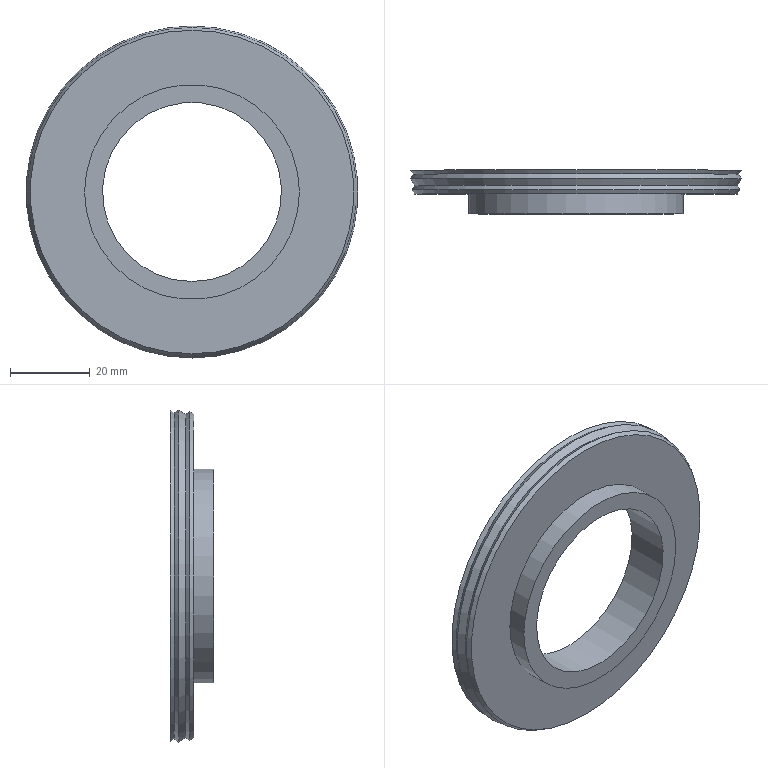Part | NX | features DATUM_CSYS 5, SKETCH 4, EXTRUDE 3, SWP104 1 | 1 solid | 10 faces | box 83.468 x 11 x 83.468 mm | volume 25904 mm3 | cone 5 | plane 3 | cylinder 2 | commonest cylinder face diameters 45 x1 54 x1
STEP:
#1=CARTESIAN_POINT('',(27.,-6.,0.));
#2=VERTEX_POINT('',#1);
#3=CARTESIAN_POINT('',(0.,-6.,0.));
#4=DIRECTION('',(0.,-1.,0.));
#5=DIRECTION('',(1.,0.,0.));
#6=AXIS2_PLACEMENT_3D('',#3,#4,#5);
#7=CIRCLE('',#6,27.);
#8=EDGE_CURVE('',#2,#2,#7,.T.);
#9=ORIENTED_EDGE('',*,*,#8,.F.);
#10=EDGE_LOOP('',(#9));
#11=FACE_BOUND('',#10,.T.);
#12=CARTESIAN_POINT('',(0.,-6.,-40.661));
#13=VERTEX_POINT('',#12);
#14=CARTESIAN_POINT('',(0.,-6.,0.));
#15=DIRECTION('',(0.,-1.,0.));
#16=DIRECTION('',(0.,0.,-1.));
#17=AXIS2_PLACEMENT_3D('',#14,#15,#16);
#18=CIRCLE('',#17,40.661);
#19=EDGE_CURVE('',#13,#13,#18,.T.);
#20=ORIENTED_EDGE('',*,*,#19,.T.);
#21=EDGE_LOOP('',(#20));
#22=FACE_BOUND('',#21,.T.);
#23=CARTESIAN_POINT('',(0.,-6.,0.));
#24=DIRECTION('',(0.,-1.,0.));
#25=DIRECTION('',(0.,0.,-1.));
#26=AXIS2_PLACEMENT_3D('',#23,#24,#25);
#27=PLANE('',#26);
#28=ADVANCED_FACE('',(#11,#22),#27,.T.);
#29=CARTESIAN_POINT('',(27.,-11.,0.));
#30=VERTEX_POINT('',#29);
#31=CARTESIAN_POINT('',(0.,-11.,0.));
#32=DIRECTION('',(0.,-1.,0.));
#33=DIRECTION('',(1.,0.,0.));
#34=AXIS2_PLACEMENT_3D('',#31,#32,#33);
#35=CIRCLE('',#34,27.);
#36=EDGE_CURVE('',#30,#30,#35,.T.);
#37=ORIENTED_EDGE('',*,*,#36,.F.);
#38=EDGE_LOOP('',(#37));
#39=FACE_BOUND('',#38,.T.);
#40=ORIENTED_EDGE('',*,*,#8,.T.);
#41=EDGE_LOOP('',(#40));
#42=FACE_BOUND('',#41,.T.);
#43=CARTESIAN_POINT('',(0.,-11.,0.));
#44=DIRECTION('',(0.,1.,0.));
#45=DIRECTION('',(0.,0.,1.));
#46=AXIS2_PLACEMENT_3D('',#43,#44,#45);
#47=CYLINDRICAL_SURFACE('',#46,27.);
#48=ADVANCED_FACE('',(#39,#42),#47,.T.);
#49=CARTESIAN_POINT('',(0.,-11.,-22.5));
#50=VERTEX_POINT('',#49);
#51=CARTESIAN_POINT('',(0.,-11.,0.));
#52=DIRECTION('',(0.,-1.,0.));
#53=DIRECTION('',(0.,0.,-1.));
#54=AXIS2_PLACEMENT_3D('',#51,#52,#53);
#55=CIRCLE('',#54,22.5);
#56=EDGE_CURVE('',#50,#50,#55,.F.);
#57=ORIENTED_EDGE('',*,*,#56,.T.);
#58=EDGE_LOOP('',(#57));
#59=FACE_BOUND('',#58,.T.);
#60=ORIENTED_EDGE('',*,*,#36,.T.);
#61=EDGE_LOOP('',(#60));
#62=FACE_BOUND('',#61,.T.);
#63=CARTESIAN_POINT('',(0.,-11.,0.));
#64=DIRECTION('',(0.,-1.,0.));
#65=DIRECTION('',(0.,0.,-1.));
#66=AXIS2_PLACEMENT_3D('',#63,#64,#65);
#67=PLANE('',#66);
#68=ADVANCED_FACE('',(#59,#62),#67,.T.);
#69=CARTESIAN_POINT('',(0.,-1.,-41.));
#70=VERTEX_POINT('',#69);
#71=CARTESIAN_POINT('',(0.,-1.,0.));
#72=DIRECTION('',(0.,-1.,0.));
#73=DIRECTION('',(0.,0.,-1.));
#74=AXIS2_PLACEMENT_3D('',#71,#72,#73);
#75=CIRCLE('',#74,41.);
#76=EDGE_CURVE('',#70,#70,#75,.F.);
#77=ORIENTED_EDGE('',*,*,#76,.T.);
#78=EDGE_LOOP('',(#77));
#79=FACE_BOUND('',#78,.T.);
#80=CARTESIAN_POINT('',(0.,0.,-41.623));
#81=VERTEX_POINT('',#80);
#82=CARTESIAN_POINT('',(0.,0.,0.));
#83=DIRECTION('',(0.,-1.,0.));
#84=DIRECTION('',(0.,0.,-1.));
#85=AXIS2_PLACEMENT_3D('',#82,#83,#84);
#86=CIRCLE('',#85,41.623);
#87=EDGE_CURVE('',#81,#81,#86,.T.);
#88=ORIENTED_EDGE('',*,*,#87,.T.);
#89=EDGE_LOOP('',(#88));
#90=FACE_BOUND('',#89,.T.);
#91=CARTESIAN_POINT('',(0.,-1.,0.));
#92=DIRECTION('',(0.,1.,0.));
#93=DIRECTION('',(0.,0.,1.));
#94=AXIS2_PLACEMENT_3D('',#91,#92,#93);
#95=CONICAL_SURFACE('',#94,41.,0.5574);
#96=ADVANCED_FACE('',(#79,#90),#95,.T.);
#97=ORIENTED_EDGE('',*,*,#19,.F.);
#98=EDGE_LOOP('',(#97));
#99=FACE_BOUND('',#98,.T.);
#100=CARTESIAN_POINT('',(0.,-4.953,-41.314));
#101=VERTEX_POINT('',#100);
#102=CARTESIAN_POINT('',(0.,-4.953,0.));
#103=DIRECTION('',(0.,-1.,0.));
#104=DIRECTION('',(0.,0.,-1.));
#105=AXIS2_PLACEMENT_3D('',#102,#103,#104);
#106=CIRCLE('',#105,41.314);
#107=EDGE_CURVE('',#101,#101,#106,.F.);
#108=ORIENTED_EDGE('',*,*,#107,.F.);
#109=EDGE_LOOP('',(#108));
#110=FACE_BOUND('',#109,.T.);
#111=CARTESIAN_POINT('',(0.,-6.121,0.));
#112=DIRECTION('',(0.,1.,0.));
#113=DIRECTION('',(0.,0.,1.));
#114=AXIS2_PLACEMENT_3D('',#111,#112,#113);
#115=CONICAL_SURFACE('',#114,40.586,0.5574);
#116=ADVANCED_FACE('',(#99,#110),#115,.T.);
#117=CARTESIAN_POINT('',(0.,-3.9,-40.631));
#118=VERTEX_POINT('',#117);
#119=CARTESIAN_POINT('',(0.,-3.9,0.));
#120=DIRECTION('',(0.,-1.,0.));
#121=DIRECTION('',(0.,0.,-1.));
#122=AXIS2_PLACEMENT_3D('',#119,#120,#121);
#123=CIRCLE('',#122,40.631);
#124=EDGE_CURVE('',#118,#118,#123,.F.);
#125=ORIENTED_EDGE('',*,*,#124,.F.);
#126=EDGE_LOOP('',(#125));
#127=FACE_BOUND('',#126,.T.);
#128=ORIENTED_EDGE('',*,*,#107,.T.);
#129=EDGE_LOOP('',(#128));
#130=FACE_BOUND('',#129,.T.);
#131=CARTESIAN_POINT('',(0.,-4.953,0.));
#132=DIRECTION('',(0.,-1.,0.));
#133=DIRECTION('',(0.,0.,-1.));
#134=AXIS2_PLACEMENT_3D('',#131,#132,#133);
#135=CONICAL_SURFACE('',#134,41.314,0.5756);
#136=ADVANCED_FACE('',(#127,#130),#135,.T.);
#137=CARTESIAN_POINT('',(0.,-2.131,-41.734));
#138=VERTEX_POINT('',#137);
#139=CARTESIAN_POINT('',(0.,-2.131,0.));
#140=DIRECTION('',(0.,-1.,0.));
#141=DIRECTION('',(0.,0.,-1.));
#142=AXIS2_PLACEMENT_3D('',#139,#140,#141);
#143=CIRCLE('',#142,41.734);
#144=EDGE_CURVE('',#138,#138,#143,.F.);
#145=ORIENTED_EDGE('',*,*,#144,.F.);
#146=EDGE_LOOP('',(#145));
#147=FACE_BOUND('',#146,.T.);
#148=ORIENTED_EDGE('',*,*,#124,.T.);
#149=EDGE_LOOP('',(#148));
#150=FACE_BOUND('',#149,.T.);
#151=CARTESIAN_POINT('',(0.,-3.9,0.));
#152=DIRECTION('',(0.,1.,0.));
#153=DIRECTION('',(0.,0.,1.));
#154=AXIS2_PLACEMENT_3D('',#151,#152,#153);
#155=CONICAL_SURFACE('',#154,40.631,0.5574);
#156=ADVANCED_FACE('',(#147,#150),#155,.T.);
#157=ORIENTED_EDGE('',*,*,#76,.F.);
#158=EDGE_LOOP('',(#157));
#159=FACE_BOUND('',#158,.T.);
#160=ORIENTED_EDGE('',*,*,#144,.T.);
#161=EDGE_LOOP('',(#160));
#162=FACE_BOUND('',#161,.T.);
#163=CARTESIAN_POINT('',(0.,-2.131,0.));
#164=DIRECTION('',(0.,-1.,0.));
#165=DIRECTION('',(0.,0.,-1.));
#166=AXIS2_PLACEMENT_3D('',#163,#164,#165);
#167=CONICAL_SURFACE('',#166,41.734,0.5756);
#168=ADVANCED_FACE('',(#159,#162),#167,.T.);
#169=CARTESIAN_POINT('',(0.,0.,-22.5));
#170=VERTEX_POINT('',#169);
#171=CARTESIAN_POINT('',(0.,0.,0.));
#172=DIRECTION('',(0.,-1.,0.));
#173=DIRECTION('',(0.,0.,-1.));
#174=AXIS2_PLACEMENT_3D('',#171,#172,#173);
#175=CIRCLE('',#174,22.5);
#176=EDGE_CURVE('',#170,#170,#175,.F.);
#177=ORIENTED_EDGE('',*,*,#176,.F.);
#178=EDGE_LOOP('',(#177));
#179=FACE_BOUND('',#178,.T.);
#180=ORIENTED_EDGE('',*,*,#87,.F.);
#181=EDGE_LOOP('',(#180));
#182=FACE_BOUND('',#181,.T.);
#183=CARTESIAN_POINT('',(0.,0.,0.));
#184=DIRECTION('',(0.,-1.,0.));
#185=DIRECTION('',(0.,0.,-1.));
#186=AXIS2_PLACEMENT_3D('',#183,#184,#185);
#187=PLANE('',#186);
#188=ADVANCED_FACE('',(#179,#182),#187,.F.);
#189=ORIENTED_EDGE('',*,*,#56,.F.);
#190=EDGE_LOOP('',(#189));
#191=FACE_BOUND('',#190,.T.);
#192=ORIENTED_EDGE('',*,*,#176,.T.);
#193=EDGE_LOOP('',(#192));
#194=FACE_BOUND('',#193,.T.);
#195=CARTESIAN_POINT('',(0.,-28.,0.));
#196=DIRECTION('',(0.,1.,0.));
#197=DIRECTION('',(0.,0.,1.));
#198=AXIS2_PLACEMENT_3D('',#195,#196,#197);
#199=CYLINDRICAL_SURFACE('',#198,22.5);
#200=ADVANCED_FACE('',(#191,#194),#199,.F.);
#201=CLOSED_SHELL('',(#28,#48,#68,#96,#116,#136,#156,#168,#188,#200));
#202=MANIFOLD_SOLID_BREP('',#201);
#203=(LENGTH_UNIT()NAMED_UNIT(*)SI_UNIT(.MILLI.,.METRE.));
#204=UNCERTAINTY_MEASURE_WITH_UNIT(LENGTH_MEASURE(0.00001),#203,'','');
#205=(NAMED_UNIT(*)PLANE_ANGLE_UNIT()SI_UNIT($,.RADIAN.));
#206=(NAMED_UNIT(*)SI_UNIT($,.STERADIAN.)SOLID_ANGLE_UNIT());
#207=(GEOMETRIC_REPRESENTATION_CONTEXT(3)GLOBAL_UNCERTAINTY_ASSIGNED_CONTEXT((#204))GLOBAL_UNIT_ASSIGNED_CONTEXT((#203,#205,#206))REPRESENTATION_CONTEXT('',''));
#208=ADVANCED_BREP_SHAPE_REPRESENTATION('',(#202),#207);